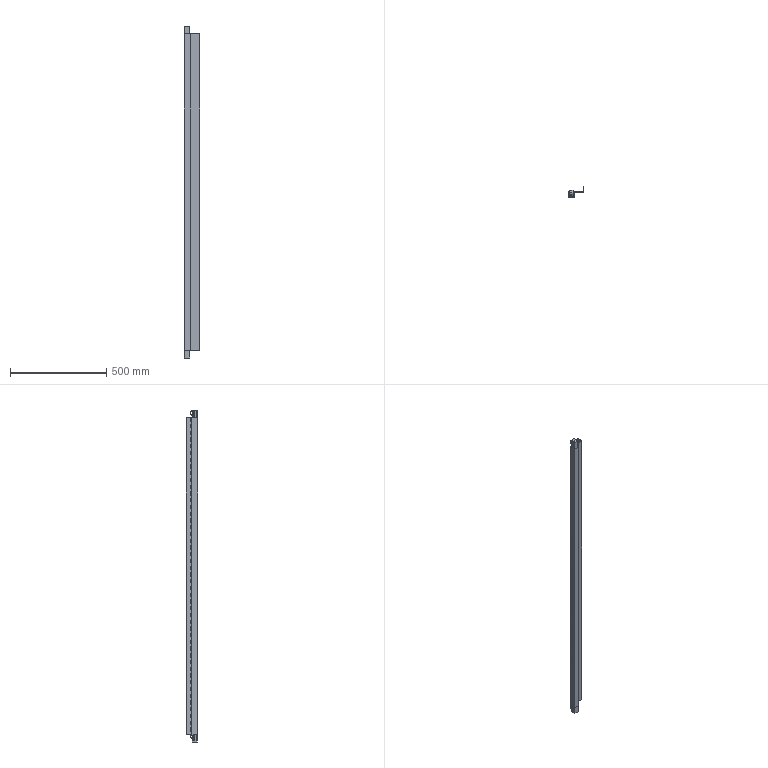Part | STEP file | Rieles | 75 solids | 2332 faces | box 81.4 x 57.7 x 1724 mm | volume 936663 mm3 | cylinder 1150 | plane 982 | spline 200 | commonest cylinder face diameters 10 x392 25 x392 4 x154 5 x98 30 x98 1.473 x8